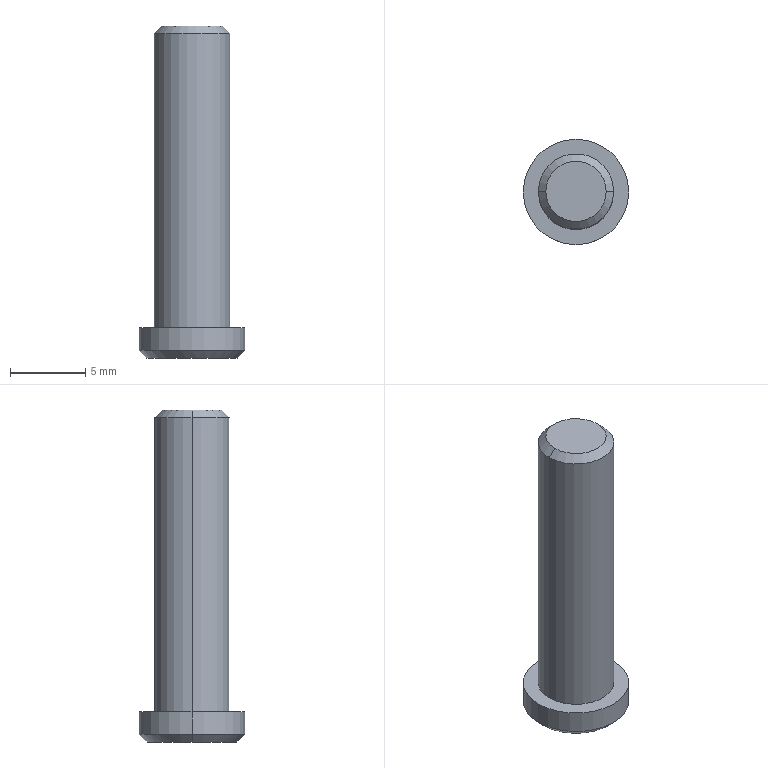Part | NX | features BREP 1 | 1 solid | 11 faces | box 7 x 7 x 22 mm | volume 465.218 mm3 | cone 4 | cylinder 4 | plane 3 | commonest cylinder face diameters 5 x2 7 x2
STEP:
#1=CARTESIAN_POINT('',(2.,0.,10.));
#2=VERTEX_POINT('',#1);
#3=CARTESIAN_POINT('',(-2.,0.,10.));
#4=VERTEX_POINT('',#3);
#5=CARTESIAN_POINT('',(0.,0.,10.));
#6=DIRECTION('',(0.,0.,1.));
#7=DIRECTION('',(1.,0.,0.));
#8=AXIS2_PLACEMENT_3D('',#5,#6,#7);
#9=CIRCLE('',#8,2.);
#10=EDGE_CURVE('',#2,#4,#9,.T.);
#11=ORIENTED_EDGE('',*,*,#10,.F.);
#12=CARTESIAN_POINT('',(2.5,0.,9.5));
#13=VERTEX_POINT('',#12);
#14=CARTESIAN_POINT('',(2.,0.,10.));
#15=DIRECTION('',(0.7071,0.,-0.7071));
#16=VECTOR('',#15,1000.);
#17=LINE('',#14,#16);
#18=EDGE_CURVE('',#2,#13,#17,.T.);
#19=ORIENTED_EDGE('',*,*,#18,.T.);
#20=CARTESIAN_POINT('',(-2.5,0.,9.5));
#21=VERTEX_POINT('',#20);
#22=CARTESIAN_POINT('',(0.,0.,9.5));
#23=DIRECTION('',(0.,0.,-1.));
#24=DIRECTION('',(1.,0.,0.));
#25=AXIS2_PLACEMENT_3D('',#22,#23,#24);
#26=CIRCLE('',#25,2.5);
#27=EDGE_CURVE('',#21,#13,#26,.T.);
#28=ORIENTED_EDGE('',*,*,#27,.F.);
#29=CARTESIAN_POINT('',(-2.,0.,10.));
#30=DIRECTION('',(-0.7071,0.,-0.7071));
#31=VECTOR('',#30,1000.);
#32=LINE('',#29,#31);
#33=EDGE_CURVE('',#4,#21,#32,.T.);
#34=ORIENTED_EDGE('',*,*,#33,.F.);
#35=EDGE_LOOP('',(#11,#19,#28,#34));
#36=FACE_BOUND('',#35,.T.);
#37=CARTESIAN_POINT('',(0.,0.,10.));
#38=DIRECTION('',(0.,0.,-1.));
#39=DIRECTION('',(-1.,0.,0.));
#40=AXIS2_PLACEMENT_3D('',#37,#38,#39);
#41=CONICAL_SURFACE('',#40,2.,0.7854);
#42=ADVANCED_FACE('',(#36),#41,.T.);
#43=CARTESIAN_POINT('',(-3.,0.,-12.));
#44=VERTEX_POINT('',#43);
#45=CARTESIAN_POINT('',(3.,0.,-12.));
#46=VERTEX_POINT('',#45);
#47=CARTESIAN_POINT('',(0.,0.,-12.));
#48=DIRECTION('',(0.,0.,-1.));
#49=DIRECTION('',(-1.,0.,0.));
#50=AXIS2_PLACEMENT_3D('',#47,#48,#49);
#51=CIRCLE('',#50,3.);
#52=EDGE_CURVE('',#44,#46,#51,.T.);
#53=ORIENTED_EDGE('',*,*,#52,.F.);
#54=CARTESIAN_POINT('',(-3.5,0.,-11.5));
#55=VERTEX_POINT('',#54);
#56=CARTESIAN_POINT('',(-3.,0.,-12.));
#57=DIRECTION('',(-0.7071,0.,0.7071));
#58=VECTOR('',#57,1000.);
#59=LINE('',#56,#58);
#60=EDGE_CURVE('',#55,#44,#59,.F.);
#61=ORIENTED_EDGE('',*,*,#60,.F.);
#62=CARTESIAN_POINT('',(3.5,0.,-11.5));
#63=VERTEX_POINT('',#62);
#64=CARTESIAN_POINT('',(0.,0.,-11.5));
#65=DIRECTION('',(0.,0.,1.));
#66=DIRECTION('',(-1.,0.,0.));
#67=AXIS2_PLACEMENT_3D('',#64,#65,#66);
#68=CIRCLE('',#67,3.5);
#69=EDGE_CURVE('',#63,#55,#68,.T.);
#70=ORIENTED_EDGE('',*,*,#69,.F.);
#71=CARTESIAN_POINT('',(3.,0.,-12.));
#72=DIRECTION('',(0.7071,0.,0.7071));
#73=VECTOR('',#72,1000.);
#74=LINE('',#71,#73);
#75=EDGE_CURVE('',#63,#46,#74,.F.);
#76=ORIENTED_EDGE('',*,*,#75,.T.);
#77=EDGE_LOOP('',(#53,#61,#70,#76));
#78=FACE_BOUND('',#77,.T.);
#79=CARTESIAN_POINT('',(0.,0.,-12.));
#80=DIRECTION('',(0.,0.,1.));
#81=DIRECTION('',(1.,0.,0.));
#82=AXIS2_PLACEMENT_3D('',#79,#80,#81);
#83=CONICAL_SURFACE('',#82,3.,0.7854);
#84=ADVANCED_FACE('',(#78),#83,.T.);
#85=ORIENTED_EDGE('',*,*,#69,.T.);
#86=CARTESIAN_POINT('',(-3.5,0.,-10.));
#87=VERTEX_POINT('',#86);
#88=CARTESIAN_POINT('',(-3.5,0.,-12.));
#89=DIRECTION('',(0.,0.,1.));
#90=VECTOR('',#89,1000.);
#91=LINE('',#88,#90);
#92=EDGE_CURVE('',#87,#55,#91,.F.);
#93=ORIENTED_EDGE('',*,*,#92,.F.);
#94=CARTESIAN_POINT('',(3.5,0.,-10.));
#95=VERTEX_POINT('',#94);
#96=CARTESIAN_POINT('',(0.,0.,-10.));
#97=DIRECTION('',(0.,0.,-1.));
#98=DIRECTION('',(-1.,0.,0.));
#99=AXIS2_PLACEMENT_3D('',#96,#97,#98);
#100=CIRCLE('',#99,3.5);
#101=EDGE_CURVE('',#87,#95,#100,.T.);
#102=ORIENTED_EDGE('',*,*,#101,.T.);
#103=CARTESIAN_POINT('',(3.5,0.,-12.));
#104=DIRECTION('',(0.,0.,1.));
#105=VECTOR('',#104,1000.);
#106=LINE('',#103,#105);
#107=EDGE_CURVE('',#95,#63,#106,.F.);
#108=ORIENTED_EDGE('',*,*,#107,.T.);
#109=EDGE_LOOP('',(#85,#93,#102,#108));
#110=FACE_BOUND('',#109,.T.);
#111=CARTESIAN_POINT('',(0.,0.,-12.));
#112=DIRECTION('',(0.,0.,1.));
#113=DIRECTION('',(1.,0.,0.));
#114=AXIS2_PLACEMENT_3D('',#111,#112,#113);
#115=CYLINDRICAL_SURFACE('',#114,3.5);
#116=ADVANCED_FACE('',(#110),#115,.T.);
#117=CARTESIAN_POINT('',(2.5,0.,-10.));
#118=VERTEX_POINT('',#117);
#119=CARTESIAN_POINT('',(-2.5,0.,-10.));
#120=VERTEX_POINT('',#119);
#121=CARTESIAN_POINT('',(0.,0.,-10.));
#122=DIRECTION('',(0.,0.,1.));
#123=DIRECTION('',(-1.,0.,0.));
#124=AXIS2_PLACEMENT_3D('',#121,#122,#123);
#125=CIRCLE('',#124,2.5);
#126=EDGE_CURVE('',#118,#120,#125,.T.);
#127=ORIENTED_EDGE('',*,*,#126,.T.);
#128=CARTESIAN_POINT('',(-2.5,0.,0.));
#129=DIRECTION('',(0.,0.,1.));
#130=VECTOR('',#129,1000.);
#131=LINE('',#128,#130);
#132=EDGE_CURVE('',#21,#120,#131,.F.);
#133=ORIENTED_EDGE('',*,*,#132,.F.);
#134=ORIENTED_EDGE('',*,*,#27,.T.);
#135=CARTESIAN_POINT('',(2.5,0.,0.));
#136=DIRECTION('',(0.,0.,1.));
#137=VECTOR('',#136,1000.);
#138=LINE('',#135,#137);
#139=EDGE_CURVE('',#13,#118,#138,.F.);
#140=ORIENTED_EDGE('',*,*,#139,.T.);
#141=EDGE_LOOP('',(#127,#133,#134,#140));
#142=FACE_BOUND('',#141,.T.);
#143=CARTESIAN_POINT('',(0.,0.,0.));
#144=DIRECTION('',(0.,0.,1.));
#145=DIRECTION('',(1.,0.,0.));
#146=AXIS2_PLACEMENT_3D('',#143,#144,#145);
#147=CYLINDRICAL_SURFACE('',#146,2.5);
#148=ADVANCED_FACE('',(#142),#147,.T.);
#149=ORIENTED_EDGE('',*,*,#132,.T.);
#150=CARTESIAN_POINT('',(0.,0.,-10.));
#151=DIRECTION('',(0.,0.,1.));
#152=DIRECTION('',(-1.,0.,0.));
#153=AXIS2_PLACEMENT_3D('',#150,#151,#152);
#154=CIRCLE('',#153,2.5);
#155=EDGE_CURVE('',#120,#118,#154,.T.);
#156=ORIENTED_EDGE('',*,*,#155,.T.);
#157=ORIENTED_EDGE('',*,*,#139,.F.);
#158=CARTESIAN_POINT('',(0.,0.,9.5));
#159=DIRECTION('',(0.,0.,-1.));
#160=DIRECTION('',(1.,0.,0.));
#161=AXIS2_PLACEMENT_3D('',#158,#159,#160);
#162=CIRCLE('',#161,2.5);
#163=EDGE_CURVE('',#13,#21,#162,.T.);
#164=ORIENTED_EDGE('',*,*,#163,.T.);
#165=EDGE_LOOP('',(#149,#156,#157,#164));
#166=FACE_BOUND('',#165,.T.);
#167=CARTESIAN_POINT('',(0.,0.,0.));
#168=DIRECTION('',(0.,0.,1.));
#169=DIRECTION('',(1.,0.,0.));
#170=AXIS2_PLACEMENT_3D('',#167,#168,#169);
#171=CYLINDRICAL_SURFACE('',#170,2.5);
#172=ADVANCED_FACE('',(#166),#171,.T.);
#173=CARTESIAN_POINT('',(0.,0.,10.));
#174=DIRECTION('',(0.,0.,1.));
#175=DIRECTION('',(1.,0.,0.));
#176=AXIS2_PLACEMENT_3D('',#173,#174,#175);
#177=CIRCLE('',#176,2.);
#178=EDGE_CURVE('',#4,#2,#177,.T.);
#179=ORIENTED_EDGE('',*,*,#178,.T.);
#180=ORIENTED_EDGE('',*,*,#10,.T.);
#181=EDGE_LOOP('',(#179,#180));
#182=FACE_BOUND('',#181,.T.);
#183=CARTESIAN_POINT('',(0.,0.,10.));
#184=DIRECTION('',(0.,0.,1.));
#185=DIRECTION('',(1.,0.,0.));
#186=AXIS2_PLACEMENT_3D('',#183,#184,#185);
#187=PLANE('',#186);
#188=ADVANCED_FACE('',(#182),#187,.T.);
#189=ORIENTED_EDGE('',*,*,#92,.T.);
#190=CARTESIAN_POINT('',(0.,0.,-11.5));
#191=DIRECTION('',(0.,0.,1.));
#192=DIRECTION('',(-1.,0.,0.));
#193=AXIS2_PLACEMENT_3D('',#190,#191,#192);
#194=CIRCLE('',#193,3.5);
#195=EDGE_CURVE('',#55,#63,#194,.T.);
#196=ORIENTED_EDGE('',*,*,#195,.T.);
#197=ORIENTED_EDGE('',*,*,#107,.F.);
#198=CARTESIAN_POINT('',(0.,0.,-10.));
#199=DIRECTION('',(0.,0.,-1.));
#200=DIRECTION('',(-1.,0.,0.));
#201=AXIS2_PLACEMENT_3D('',#198,#199,#200);
#202=CIRCLE('',#201,3.5);
#203=EDGE_CURVE('',#95,#87,#202,.T.);
#204=ORIENTED_EDGE('',*,*,#203,.T.);
#205=EDGE_LOOP('',(#189,#196,#197,#204));
#206=FACE_BOUND('',#205,.T.);
#207=CARTESIAN_POINT('',(0.,0.,-12.));
#208=DIRECTION('',(0.,0.,1.));
#209=DIRECTION('',(1.,0.,0.));
#210=AXIS2_PLACEMENT_3D('',#207,#208,#209);
#211=CYLINDRICAL_SURFACE('',#210,3.5);
#212=ADVANCED_FACE('',(#206),#211,.T.);
#213=CARTESIAN_POINT('',(0.,0.,-12.));
#214=DIRECTION('',(0.,0.,-1.));
#215=DIRECTION('',(-1.,0.,0.));
#216=AXIS2_PLACEMENT_3D('',#213,#214,#215);
#217=CIRCLE('',#216,3.);
#218=EDGE_CURVE('',#46,#44,#217,.T.);
#219=ORIENTED_EDGE('',*,*,#218,.T.);
#220=ORIENTED_EDGE('',*,*,#52,.T.);
#221=EDGE_LOOP('',(#219,#220));
#222=FACE_BOUND('',#221,.T.);
#223=CARTESIAN_POINT('',(0.,0.,-12.));
#224=DIRECTION('',(0.,0.,-1.));
#225=DIRECTION('',(0.,-1.,0.));
#226=AXIS2_PLACEMENT_3D('',#223,#224,#225);
#227=PLANE('',#226);
#228=ADVANCED_FACE('',(#222),#227,.T.);
#229=ORIENTED_EDGE('',*,*,#203,.F.);
#230=ORIENTED_EDGE('',*,*,#101,.F.);
#231=EDGE_LOOP('',(#229,#230));
#232=FACE_BOUND('',#231,.T.);
#233=ORIENTED_EDGE('',*,*,#126,.F.);
#234=ORIENTED_EDGE('',*,*,#155,.F.);
#235=EDGE_LOOP('',(#233,#234));
#236=FACE_BOUND('',#235,.T.);
#237=CARTESIAN_POINT('',(0.,0.,-10.));
#238=DIRECTION('',(0.,0.,-1.));
#239=DIRECTION('',(0.,-1.,0.));
#240=AXIS2_PLACEMENT_3D('',#237,#238,#239);
#241=PLANE('',#240);
#242=ADVANCED_FACE('',(#232,#236),#241,.F.);
#243=ORIENTED_EDGE('',*,*,#60,.T.);
#244=ORIENTED_EDGE('',*,*,#218,.F.);
#245=ORIENTED_EDGE('',*,*,#75,.F.);
#246=ORIENTED_EDGE('',*,*,#195,.F.);
#247=EDGE_LOOP('',(#243,#244,#245,#246));
#248=FACE_BOUND('',#247,.T.);
#249=CARTESIAN_POINT('',(0.,0.,-12.));
#250=DIRECTION('',(0.,0.,1.));
#251=DIRECTION('',(1.,0.,0.));
#252=AXIS2_PLACEMENT_3D('',#249,#250,#251);
#253=CONICAL_SURFACE('',#252,3.,0.7854);
#254=ADVANCED_FACE('',(#248),#253,.T.);
#255=ORIENTED_EDGE('',*,*,#18,.F.);
#256=ORIENTED_EDGE('',*,*,#178,.F.);
#257=ORIENTED_EDGE('',*,*,#33,.T.);
#258=ORIENTED_EDGE('',*,*,#163,.F.);
#259=EDGE_LOOP('',(#255,#256,#257,#258));
#260=FACE_BOUND('',#259,.T.);
#261=CARTESIAN_POINT('',(0.,0.,10.));
#262=DIRECTION('',(0.,0.,-1.));
#263=DIRECTION('',(-1.,0.,0.));
#264=AXIS2_PLACEMENT_3D('',#261,#262,#263);
#265=CONICAL_SURFACE('',#264,2.,0.7854);
#266=ADVANCED_FACE('',(#260),#265,.T.);
#267=CLOSED_SHELL('',(#42,#84,#116,#148,#172,#188,#212,#228,#242,#254,#266));
#268=MANIFOLD_SOLID_BREP('',#267);
#269=(LENGTH_UNIT()NAMED_UNIT(*)SI_UNIT(.MILLI.,.METRE.));
#270=UNCERTAINTY_MEASURE_WITH_UNIT(LENGTH_MEASURE(0.00001),#269,'','');
#271=(NAMED_UNIT(*)PLANE_ANGLE_UNIT()SI_UNIT($,.RADIAN.));
#272=(NAMED_UNIT(*)SI_UNIT($,.STERADIAN.)SOLID_ANGLE_UNIT());
#273=(GEOMETRIC_REPRESENTATION_CONTEXT(3)GLOBAL_UNCERTAINTY_ASSIGNED_CONTEXT((#270))GLOBAL_UNIT_ASSIGNED_CONTEXT((#269,#271,#272))REPRESENTATION_CONTEXT('',''));
#274=ADVANCED_BREP_SHAPE_REPRESENTATION('',(#268),#273);